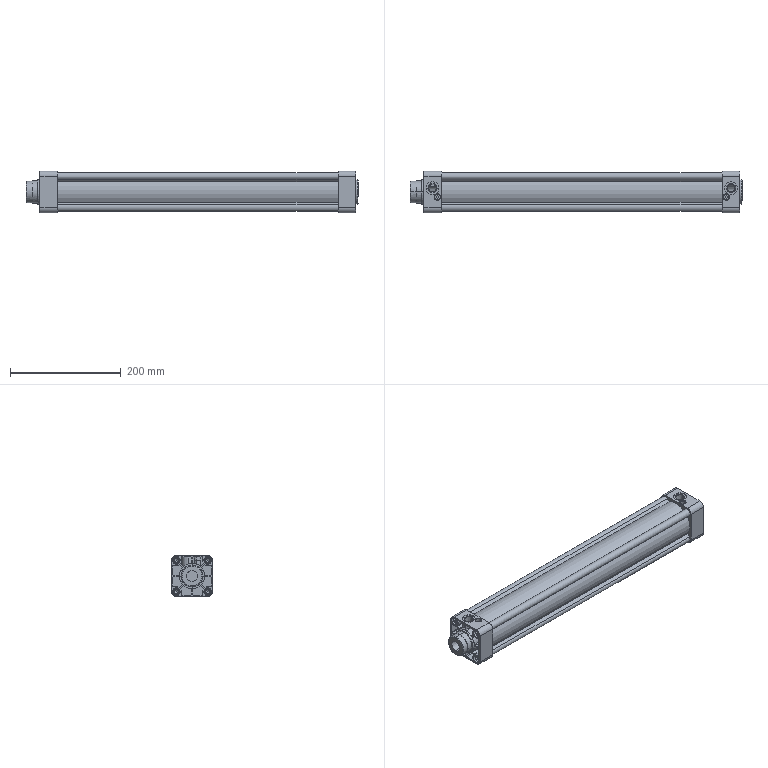Part | SolidWorks | features BaseBody 1 | 1 solid | 533 faces | box 600 x 75 x 75 mm | volume 828152 mm3 | cylinder 243 | plane 228 | cone 42 | spline 20 | commonest cylinder face diameters 3 x100 19 x20 6.647 x16 13 x16 14 x16 46 x16